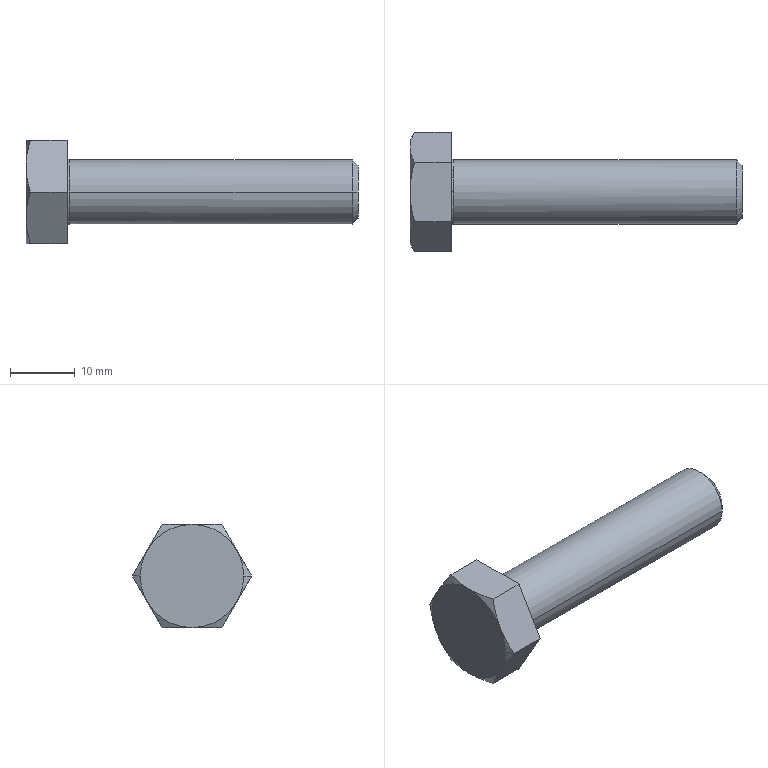Part | STEP file | KS B 1002 - C  M 10 x 45 | 1 solid | 23 faces | box 51.4 x 18.475 x 16 mm | volume 4937 mm3 | cone 10 | plane 9 | torus 2 | cylinder 2 | commonest cylinder face diameters 10 x2